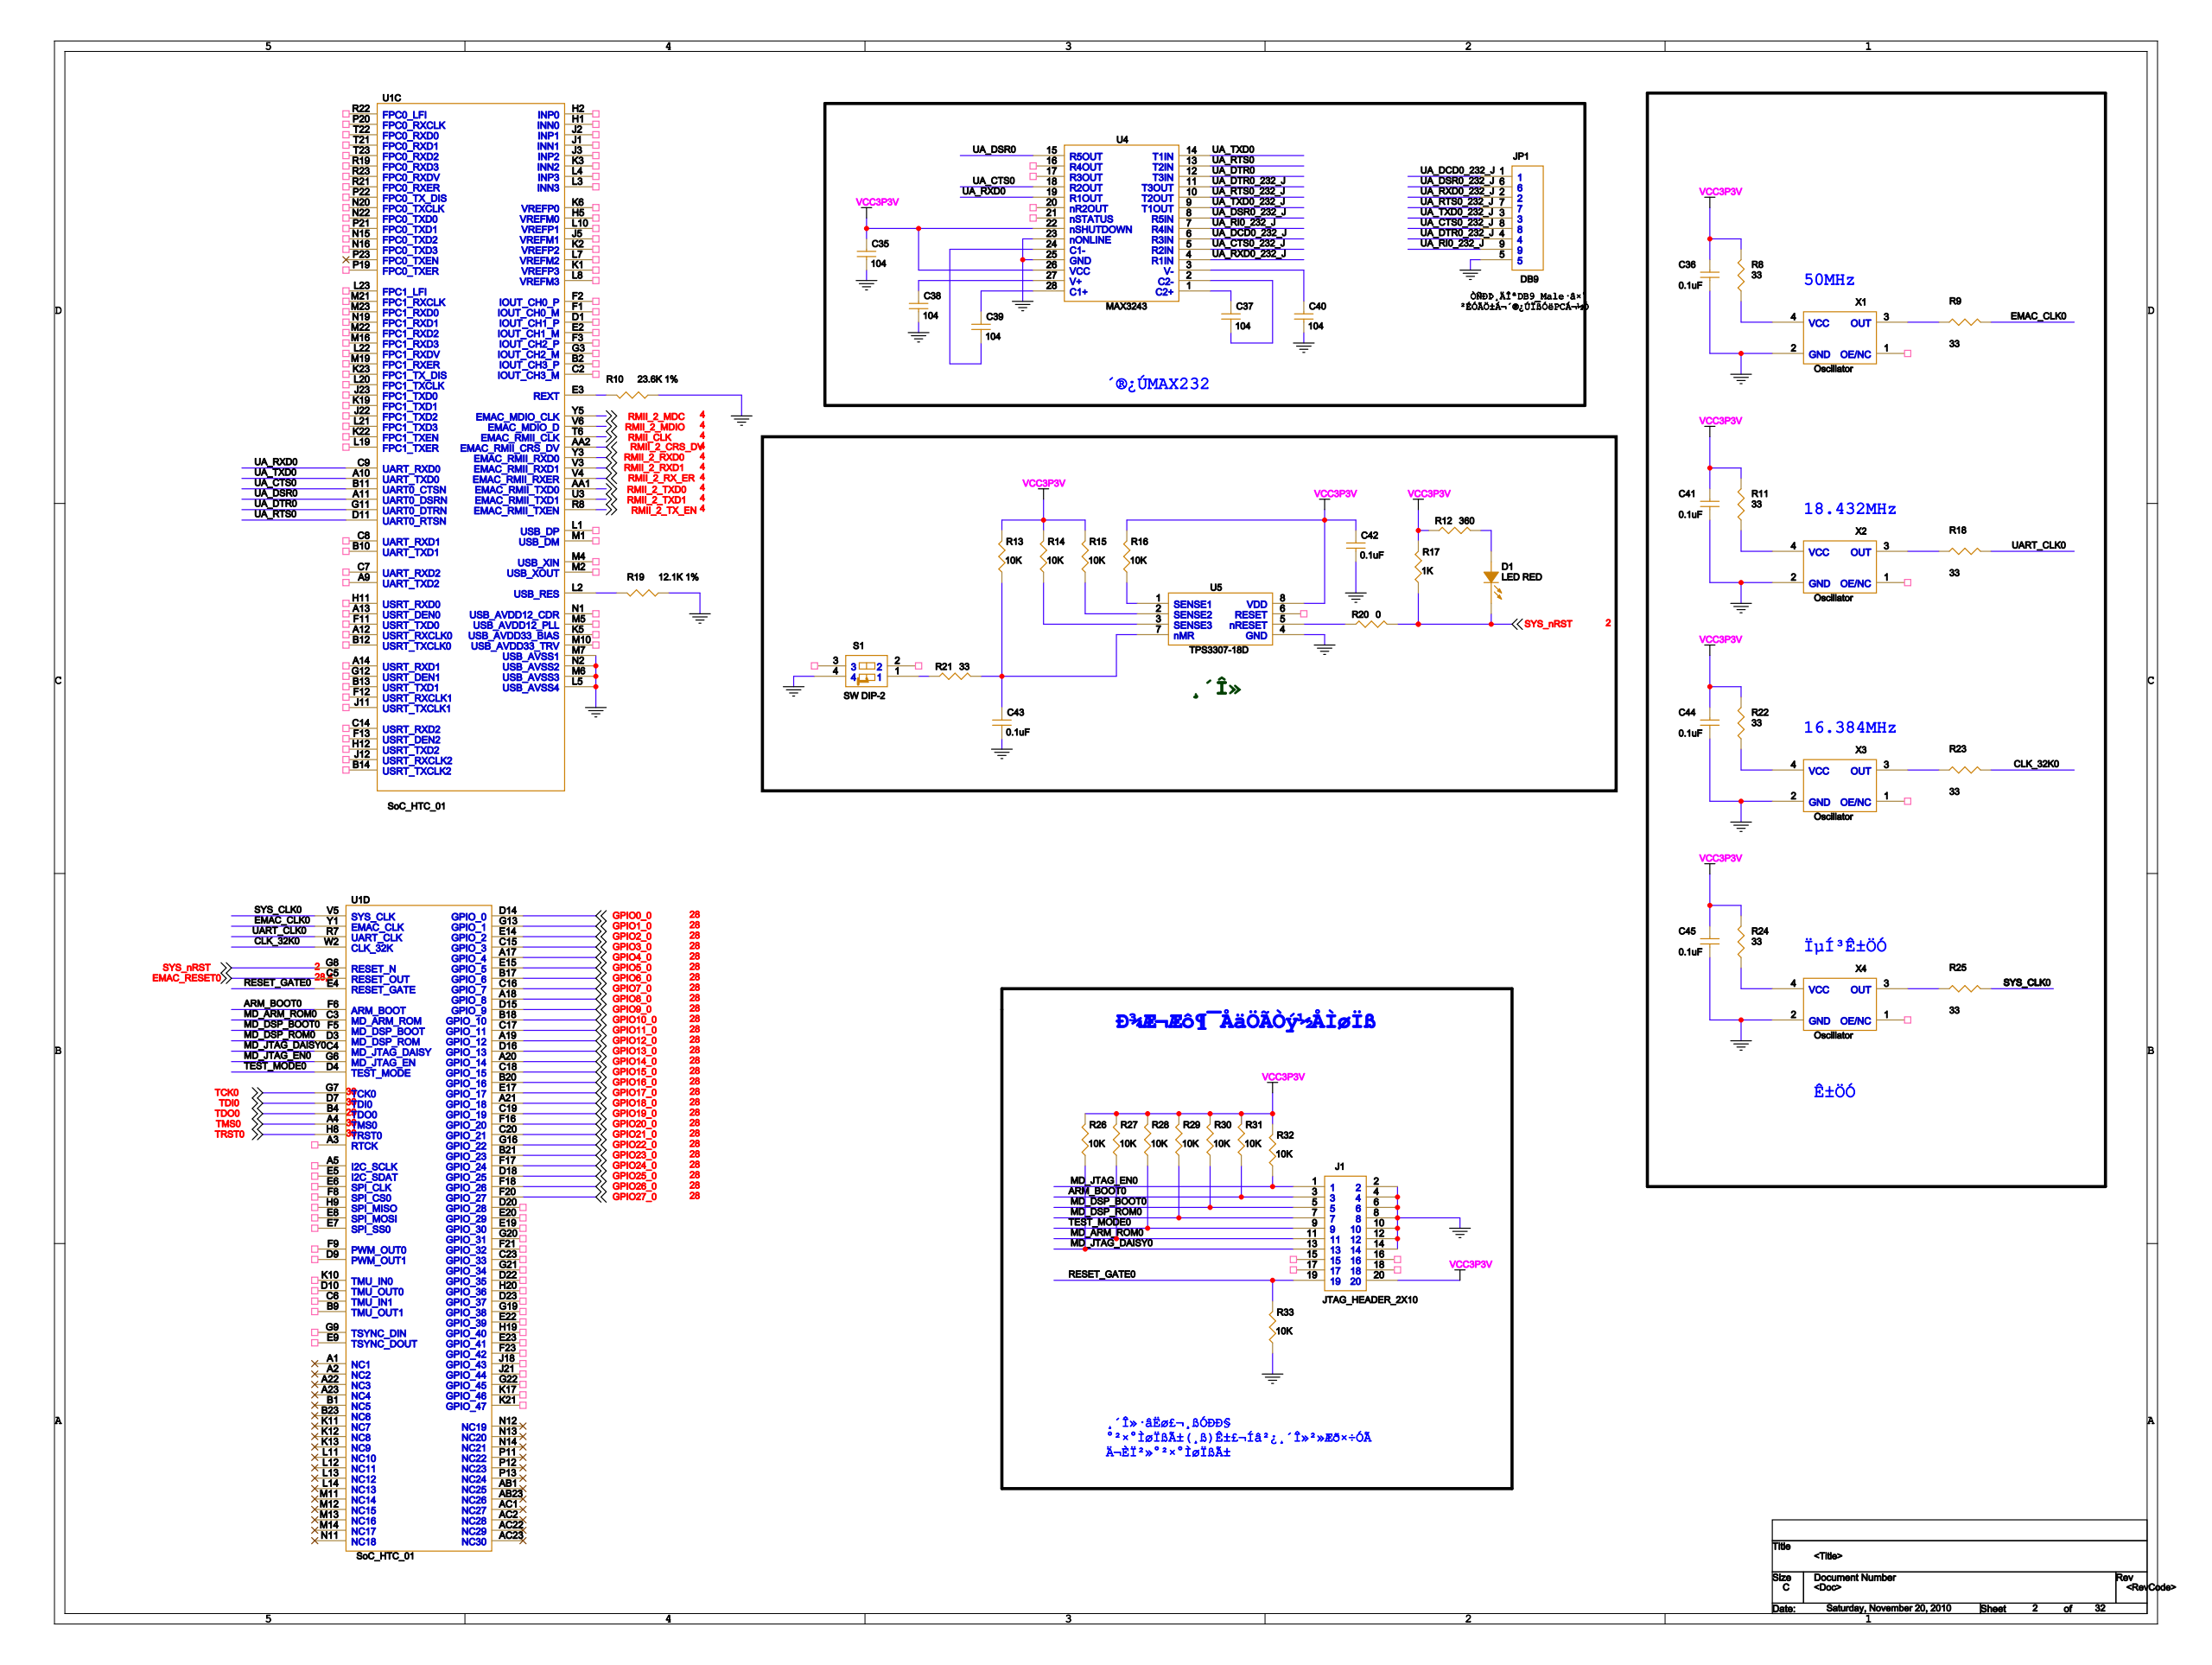Circuit board | Cadence Allegro | 1001 parts | 1318 nets | one sheet of the schematic
Parts on this sheet (reference | value | footprint):
C35 | 104 | 0603
C36 | 0.1uF | 0603
C37 | 104 | 0603
C38 | 104 | 0603
C39 | 104 | 0603
C40 | 104 | 0603
C41 | 0.1uF | 0603
C42 | 0.1uF | 0603
C43 | 0.1uF | 0603
C44 | 0.1uF | 0603
C45 | 0.1uF | 0603
J1 | JTAG_HEADER_2X10 | JTAG_HEADER_2X10
JP1 | DB9 | DB9-MALE
R9 | 33 | 0603
R12 | 360 | 0603
R17 | 1K | 0603
R18 | 33 | 0603
R20 | 0 | 0603
R23 | 33 | 0603
R26 | 10K | 0603
R27 | 10K | 0603
R28 | 10K | 0603
R29 | 10K | 0603
R30 | 10K | 0603
R31 | 10K | 0603
R32 | 10K | 0603
R33 | 10K | 0603
S1 | SW DIP-2 | SW_4
U1 | SoC_HTC_01 | L529_XIN
U4 | MAX3243 | TSSOP-28
U5 | TPS3307-18D | SO8
X1 | Oscillator | OSC_5_7
X2 | Oscillator | OSC_5_7
X3 | Oscillator | OSC_5_7
X4 | Oscillator | OSC_5_7
Nets of these parts (net: part-pin ...):
GPIO17_0: U1-E17
GPIO26_0: U1-F18
GPIO21_0: U1-C20
GPIO4_0: U1-A17
GPIO25_0: U1-D18
GPIO10_0: U1-B18
GPIO7_0: U1-C16
GPIO27_0: U1-F20
GPIO8_0: U1-A18
GPIO6_0: U1-B17
GPIO13_0: U1-D16
GPIO19_0: U1-C19
GPIO12_0: U1-A19
GPIO24_0: U1-F17
GPIO5_0: U1-E15
GPIO9_0: U1-D15
GPIO2_0: U1-E14
GPIO1_0: U1-G13
GPIO3_0: U1-C15
GPIO11_0: U1-C17
GPIO16_0: U1-B20
GPIO14_0: U1-A20
GPIO15_0: U1-C18
GPIO20_0: U1-F16
GPIO22_0: U1-G16
GPIO0_0: U1-D14
GPIO23_0: U1-B21
GPIO18_0: U1-A21
TRST0: U1-H8
TDI0: U1-D7
EMAC_RESET0: U1-C5
TDO0: U1-B4
TCK0: U1-G7
TMS0: U1-A4
GND: C35-2 C36-2 C38-2 C40-2 C41-2 C42-2 C43-2 C44-2 C45-2 J1-2 J1-4 J1-6 J1-8 J1-10 J1-12 J1-14 JP1-5 R33-1 S1-4 U5-4 X1-2 X2-2 X3-2 X4-2 U1-L5 U1-M6 U1-M7 U1-N2 U1-R16 U1-R18 U1-U5 U4-23 U4-25
VCC3P3V: C35-1 C36-1 C41-1 C42-1 C44-1 C45-1 J1-20 R12-1 R17-2 R26-2 R27-2 R28-2 R29-2 R30-2 R31-2 R32-2 U5-8 U1-R17 U4-22 U4-26
RMII_2_MDC: U1-Y5
RMII_2_MDIO: U1-V6
RMII_CLK: U1-T6
RMII_2_RXD0: U1-Y3
RMII_2_RXD1: U1-V3
RMII_2_RX_ER: U1-V4
RMII_2_TXD0: U1-AA1
RMII_2_TXD1: U1-U3
RMII_2_TX_EN: U1-R8
UA_CTS0: U1-B11 U4-18
UA_DSR0: U1-A11 U4-15
UA_DTR0: U1-G11 U4-12
UA_RTS0: U1-D11 U4-13
UA_RXD0: U1-C9 U4-19
UA_TXD0: U1-A10 U4-14
ARM_BOOT0: J1-3 R31-1 U1-F6
CLK_32K0: R23-2 U1-W2
EMAC_CLK0: R9-2 U1-Y1
MD_ARM_ROM0: J1-11 R27-1 U1-C3
MD_DSP_BOOT0: J1-5 R30-1 U1-F5
MD_DSP_ROM0: J1-7 R29-1 U1-D3
MD_JTAG_DAISY0: J1-13 R26-1 U1-C4
MD_JTAG_EN0: J1-1 R32-1 U1-G6
RESET_GATE0: J1-19 R33-2 U1-E4
SYS_NRST: R17-1 R20-2 U1-G8
TEST_MODE0: J1-9 R28-1 U1-D4
UART_CLK0: R18-2 U1-R7
N15953285: C43-1 U5-7
N15946754: C37-1 U4-1
N15946774: C37-2 U4-2
N15946724: C38-1 U4-27
N15946758: C39-1 U4-28
N15946704: C39-2 U4-24
N15946696: C40-1 U4-3
N15953301: R12-2
UA_DCD0_232_J: JP1-1 U4-6
UA_RXD0_232_J: JP1-2 U4-4
UA_TXD0_232_J: JP1-3 U4-9
UA_DTR0_232_J: JP1-4 U4-11
UA_DSR0_232_J: JP1-6 U4-8
UA_RTS0_232_J: JP1-7 U4-10
UA_CTS0_232_J: JP1-8 U4-5
UA_RI0_232_J: JP1-9 U4-7
N15953277: U5-2
N15953349: U5-1
N15953337: U5-3
N15953325: R20-1 U5-5
N15935148: R18-1 X2-3
N15953397: S1-1
N15935432: X3-4
N15935474: R23-1 X3-3
N15935554: X4-4
N15935588: X4-3
N15935022: X1-4
N15935062: R9-1 X1-3
N15935104: X2-4